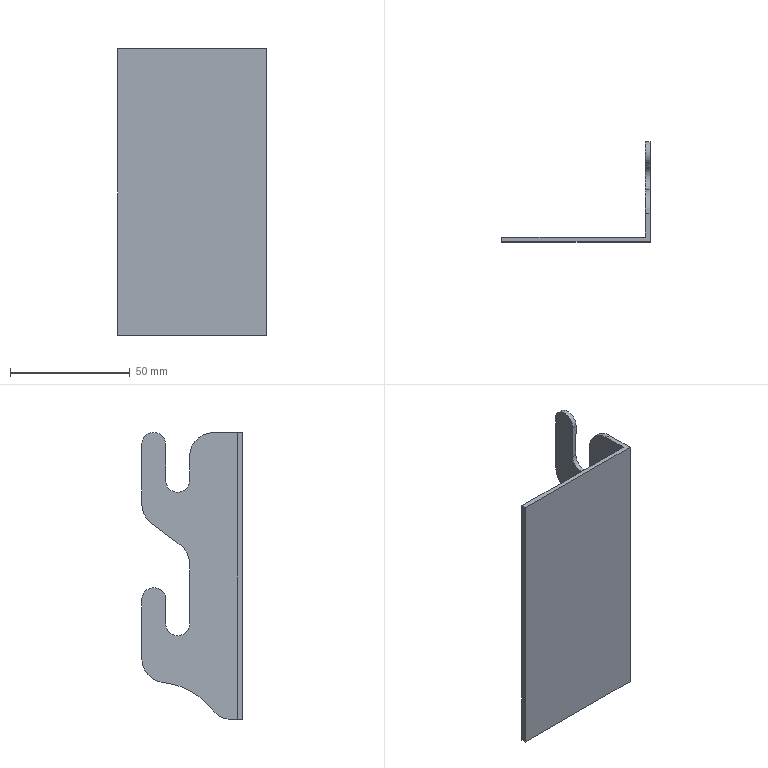Part | SolidWorks | features BaseBody 1 | 1 solid | 24 faces | box 62 x 42 x 120 mm | volume 21824 mm3 | plane 14 | cylinder 10 | commonest cylinder face diameters 20 x5 10 x3 10.188 x1 58.749 x1
STEP:
#1=CARTESIAN_POINT('',(-30.,2.,60.));
#2=VERTEX_POINT('',#1);
#3=CARTESIAN_POINT('',(30.,2.,60.));
#4=VERTEX_POINT('',#3);
#5=CARTESIAN_POINT('',(30.,2.,60.));
#6=DIRECTION('',(1.,0.,0.));
#7=VECTOR('',#6,1000.);
#8=LINE('',#5,#7);
#9=EDGE_CURVE('',#2,#4,#8,.T.);
#10=ORIENTED_EDGE('',*,*,#9,.T.);
#11=CARTESIAN_POINT('',(30.,2.,-60.));
#12=VERTEX_POINT('',#11);
#13=CARTESIAN_POINT('',(30.,2.,-60.));
#14=DIRECTION('',(0.,0.,-1.));
#15=VECTOR('',#14,1000.);
#16=LINE('',#13,#15);
#17=EDGE_CURVE('',#4,#12,#16,.T.);
#18=ORIENTED_EDGE('',*,*,#17,.T.);
#19=CARTESIAN_POINT('',(-30.,2.,-60.));
#20=VERTEX_POINT('',#19);
#21=CARTESIAN_POINT('',(-30.,2.,-60.));
#22=DIRECTION('',(-1.,0.,0.));
#23=VECTOR('',#22,1000.);
#24=LINE('',#21,#23);
#25=EDGE_CURVE('',#12,#20,#24,.T.);
#26=ORIENTED_EDGE('',*,*,#25,.T.);
#27=CARTESIAN_POINT('',(-30.,2.,60.));
#28=DIRECTION('',(0.,0.,1.));
#29=VECTOR('',#28,1000.);
#30=LINE('',#27,#29);
#31=EDGE_CURVE('',#20,#2,#30,.T.);
#32=ORIENTED_EDGE('',*,*,#31,.T.);
#33=EDGE_LOOP('',(#10,#18,#26,#32));
#34=FACE_OUTER_BOUND('',#33,.T.);
#35=CARTESIAN_POINT('',(0.,2.,0.));
#36=DIRECTION('',(0.,1.,0.));
#37=DIRECTION('',(1.,0.,0.));
#38=AXIS2_PLACEMENT_3D('',#35,#36,#37);
#39=PLANE('',#38);
#40=ADVANCED_FACE('',(#34),#39,.T.);
#41=CARTESIAN_POINT('',(32.,0.,60.));
#42=VERTEX_POINT('',#41);
#43=CARTESIAN_POINT('',(-30.,0.,60.));
#44=VERTEX_POINT('',#43);
#45=CARTESIAN_POINT('',(30.,0.,60.));
#46=DIRECTION('',(-1.,0.,0.));
#47=VECTOR('',#46,1000.);
#48=LINE('',#45,#47);
#49=EDGE_CURVE('',#42,#44,#48,.T.);
#50=ORIENTED_EDGE('',*,*,#49,.T.);
#51=CARTESIAN_POINT('',(-30.,0.,-60.));
#52=VERTEX_POINT('',#51);
#53=CARTESIAN_POINT('',(-30.,0.,60.));
#54=DIRECTION('',(0.,0.,-1.));
#55=VECTOR('',#54,1000.);
#56=LINE('',#53,#55);
#57=EDGE_CURVE('',#44,#52,#56,.T.);
#58=ORIENTED_EDGE('',*,*,#57,.T.);
#59=CARTESIAN_POINT('',(32.,0.,-60.));
#60=VERTEX_POINT('',#59);
#61=CARTESIAN_POINT('',(-30.,0.,-60.));
#62=DIRECTION('',(1.,0.,0.));
#63=VECTOR('',#62,1000.);
#64=LINE('',#61,#63);
#65=EDGE_CURVE('',#52,#60,#64,.T.);
#66=ORIENTED_EDGE('',*,*,#65,.T.);
#67=CARTESIAN_POINT('',(32.,0.,-60.));
#68=DIRECTION('',(0.,0.,-1.));
#69=VECTOR('',#68,1000.);
#70=LINE('',#67,#69);
#71=EDGE_CURVE('',#42,#60,#70,.T.);
#72=ORIENTED_EDGE('',*,*,#71,.F.);
#73=EDGE_LOOP('',(#50,#58,#66,#72));
#74=FACE_OUTER_BOUND('',#73,.T.);
#75=CARTESIAN_POINT('',(0.,0.,0.));
#76=DIRECTION('',(0.,-1.,0.));
#77=DIRECTION('',(0.,0.,-1.));
#78=AXIS2_PLACEMENT_3D('',#75,#76,#77);
#79=PLANE('',#78);
#80=ADVANCED_FACE('',(#74),#79,.T.);
#81=ORIENTED_EDGE('',*,*,#49,.F.);
#82=CARTESIAN_POINT('',(32.,12.,60.));
#83=VERTEX_POINT('',#82);
#84=CARTESIAN_POINT('',(32.,0.,60.));
#85=DIRECTION('',(0.,-1.,0.));
#86=VECTOR('',#85,1000.);
#87=LINE('',#84,#86);
#88=EDGE_CURVE('',#83,#42,#87,.T.);
#89=ORIENTED_EDGE('',*,*,#88,.F.);
#90=CARTESIAN_POINT('',(30.,12.,60.));
#91=VERTEX_POINT('',#90);
#92=CARTESIAN_POINT('',(30.,12.,60.));
#93=DIRECTION('',(1.,0.,0.));
#94=VECTOR('',#93,1000.);
#95=LINE('',#92,#94);
#96=EDGE_CURVE('',#91,#83,#95,.T.);
#97=ORIENTED_EDGE('',*,*,#96,.F.);
#98=CARTESIAN_POINT('',(30.,0.,60.));
#99=DIRECTION('',(0.,1.,0.));
#100=VECTOR('',#99,1000.);
#101=LINE('',#98,#100);
#102=EDGE_CURVE('',#4,#91,#101,.T.);
#103=ORIENTED_EDGE('',*,*,#102,.F.);
#104=ORIENTED_EDGE('',*,*,#9,.F.);
#105=CARTESIAN_POINT('',(-30.,0.,60.));
#106=DIRECTION('',(0.,1.,0.));
#107=VECTOR('',#106,1000.);
#108=LINE('',#105,#107);
#109=EDGE_CURVE('',#44,#2,#108,.T.);
#110=ORIENTED_EDGE('',*,*,#109,.F.);
#111=EDGE_LOOP('',(#81,#89,#97,#103,#104,#110));
#112=FACE_OUTER_BOUND('',#111,.T.);
#113=CARTESIAN_POINT('',(-30.,0.,60.));
#114=DIRECTION('',(0.,0.,1.));
#115=DIRECTION('',(1.,0.,0.));
#116=AXIS2_PLACEMENT_3D('',#113,#114,#115);
#117=PLANE('',#116);
#118=ADVANCED_FACE('',(#112),#117,.T.);
#119=ORIENTED_EDGE('',*,*,#65,.F.);
#120=CARTESIAN_POINT('',(-30.,0.,-60.));
#121=DIRECTION('',(0.,1.,0.));
#122=VECTOR('',#121,1000.);
#123=LINE('',#120,#122);
#124=EDGE_CURVE('',#52,#20,#123,.T.);
#125=ORIENTED_EDGE('',*,*,#124,.T.);
#126=ORIENTED_EDGE('',*,*,#25,.F.);
#127=CARTESIAN_POINT('',(30.,4.56,-60.));
#128=VERTEX_POINT('',#127);
#129=CARTESIAN_POINT('',(30.,4.56,-60.));
#130=DIRECTION('',(0.,-1.,0.));
#131=VECTOR('',#130,1000.);
#132=LINE('',#129,#131);
#133=EDGE_CURVE('',#128,#12,#132,.T.);
#134=ORIENTED_EDGE('',*,*,#133,.F.);
#135=CARTESIAN_POINT('',(32.,4.56,-60.));
#136=VERTEX_POINT('',#135);
#137=CARTESIAN_POINT('',(30.,4.56,-60.));
#138=DIRECTION('',(1.,0.,0.));
#139=VECTOR('',#138,1000.);
#140=LINE('',#137,#139);
#141=EDGE_CURVE('',#128,#136,#140,.T.);
#142=ORIENTED_EDGE('',*,*,#141,.T.);
#143=CARTESIAN_POINT('',(32.,4.56,-60.));
#144=DIRECTION('',(0.,1.,0.));
#145=VECTOR('',#144,1000.);
#146=LINE('',#143,#145);
#147=EDGE_CURVE('',#60,#136,#146,.T.);
#148=ORIENTED_EDGE('',*,*,#147,.F.);
#149=EDGE_LOOP('',(#119,#125,#126,#134,#142,#148));
#150=FACE_OUTER_BOUND('',#149,.T.);
#151=CARTESIAN_POINT('',(30.,0.,-60.));
#152=DIRECTION('',(0.,0.,-1.));
#153=DIRECTION('',(0.,-1.,0.));
#154=AXIS2_PLACEMENT_3D('',#151,#152,#153);
#155=PLANE('',#154);
#156=ADVANCED_FACE('',(#150),#155,.T.);
#157=ORIENTED_EDGE('',*,*,#57,.F.);
#158=ORIENTED_EDGE('',*,*,#109,.T.);
#159=ORIENTED_EDGE('',*,*,#31,.F.);
#160=ORIENTED_EDGE('',*,*,#124,.F.);
#161=EDGE_LOOP('',(#157,#158,#159,#160));
#162=FACE_OUTER_BOUND('',#161,.T.);
#163=CARTESIAN_POINT('',(-30.,0.,-60.));
#164=DIRECTION('',(-1.,0.,0.));
#165=DIRECTION('',(0.,1.,0.));
#166=AXIS2_PLACEMENT_3D('',#163,#164,#165);
#167=PLANE('',#166);
#168=ADVANCED_FACE('',(#162),#167,.T.);
#169=ORIENTED_EDGE('',*,*,#88,.T.);
#170=ORIENTED_EDGE('',*,*,#71,.T.);
#171=ORIENTED_EDGE('',*,*,#147,.T.);
#172=CARTESIAN_POINT('',(32.,12.53,-56.04));
#173=VERTEX_POINT('',#172);
#174=CARTESIAN_POINT('',(32.,4.56,-50.));
#175=DIRECTION('',(1.,0.,0.));
#176=DIRECTION('',(0.,0.,1.));
#177=AXIS2_PLACEMENT_3D('',#174,#175,#176);
#178=CIRCLE('',#177,10.);
#179=EDGE_CURVE('',#136,#173,#178,.T.);
#180=ORIENTED_EDGE('',*,*,#179,.T.);
#181=CARTESIAN_POINT('',(32.,33.001,-44.557));
#182=VERTEX_POINT('',#181);
#183=CARTESIAN_POINT('',(32.,35.94,-73.784));
#184=DIRECTION('',(-1.,0.,0.));
#185=DIRECTION('',(0.,-0.1001,0.995));
#186=AXIS2_PLACEMENT_3D('',#183,#184,#185);
#187=CIRCLE('',#186,29.374);
#188=EDGE_CURVE('',#173,#182,#187,.T.);
#189=ORIENTED_EDGE('',*,*,#188,.T.);
#190=CARTESIAN_POINT('',(32.,42.,-34.607));
#191=VERTEX_POINT('',#190);
#192=CARTESIAN_POINT('',(32.,32.,-34.607));
#193=DIRECTION('',(1.,0.,0.));
#194=DIRECTION('',(0.,-0.1001,0.995));
#195=AXIS2_PLACEMENT_3D('',#192,#193,#194);
#196=CIRCLE('',#195,10.);
#197=EDGE_CURVE('',#182,#191,#196,.T.);
#198=ORIENTED_EDGE('',*,*,#197,.T.);
#199=CARTESIAN_POINT('',(32.,42.,-10.));
#200=VERTEX_POINT('',#199);
#201=CARTESIAN_POINT('',(32.,42.,-10.));
#202=DIRECTION('',(0.,0.,1.));
#203=VECTOR('',#202,1000.);
#204=LINE('',#201,#203);
#205=EDGE_CURVE('',#191,#200,#204,.T.);
#206=ORIENTED_EDGE('',*,*,#205,.T.);
#207=CARTESIAN_POINT('',(32.,32.,-8.629));
#208=VERTEX_POINT('',#207);
#209=CARTESIAN_POINT('',(32.,36.906,-10.));
#210=DIRECTION('',(1.,0.,0.));
#211=DIRECTION('',(0.,-1.,0.));
#212=AXIS2_PLACEMENT_3D('',#209,#210,#211);
#213=CIRCLE('',#212,5.094);
#214=EDGE_CURVE('',#200,#208,#213,.T.);
#215=ORIENTED_EDGE('',*,*,#214,.T.);
#216=CARTESIAN_POINT('',(32.,32.,-20.));
#217=VERTEX_POINT('',#216);
#218=CARTESIAN_POINT('',(32.,32.,-20.));
#219=DIRECTION('',(0.,0.,-1.));
#220=VECTOR('',#219,1000.);
#221=LINE('',#218,#220);
#222=EDGE_CURVE('',#208,#217,#221,.T.);
#223=ORIENTED_EDGE('',*,*,#222,.T.);
#224=CARTESIAN_POINT('',(32.,22.,-20.));
#225=VERTEX_POINT('',#224);
#226=CARTESIAN_POINT('',(32.,27.,-20.));
#227=DIRECTION('',(-1.,0.,0.));
#228=DIRECTION('',(0.,-1.,0.));
#229=AXIS2_PLACEMENT_3D('',#226,#227,#228);
#230=CIRCLE('',#229,5.);
#231=EDGE_CURVE('',#217,#225,#230,.T.);
#232=ORIENTED_EDGE('',*,*,#231,.T.);
#233=CARTESIAN_POINT('',(32.,22.,5.051));
#234=VERTEX_POINT('',#233);
#235=CARTESIAN_POINT('',(32.,22.,5.051));
#236=DIRECTION('',(0.,0.,1.));
#237=VECTOR('',#236,1000.);
#238=LINE('',#235,#237);
#239=EDGE_CURVE('',#225,#234,#238,.T.);
#240=ORIENTED_EDGE('',*,*,#239,.T.);
#241=CARTESIAN_POINT('',(32.,26.,13.051));
#242=VERTEX_POINT('',#241);
#243=CARTESIAN_POINT('',(32.,32.,5.051));
#244=DIRECTION('',(-1.,0.,0.));
#245=DIRECTION('',(0.,-0.6,0.8));
#246=AXIS2_PLACEMENT_3D('',#243,#244,#245);
#247=CIRCLE('',#246,10.);
#248=EDGE_CURVE('',#234,#242,#247,.T.);
#249=ORIENTED_EDGE('',*,*,#248,.T.);
#250=CARTESIAN_POINT('',(32.,38.,22.051));
#251=VERTEX_POINT('',#250);
#252=CARTESIAN_POINT('',(32.,38.,22.051));
#253=DIRECTION('',(0.,0.8,0.6));
#254=VECTOR('',#253,1000.);
#255=LINE('',#252,#254);
#256=EDGE_CURVE('',#242,#251,#255,.T.);
#257=ORIENTED_EDGE('',*,*,#256,.T.);
#258=CARTESIAN_POINT('',(32.,42.,30.051));
#259=VERTEX_POINT('',#258);
#260=CARTESIAN_POINT('',(32.,32.,30.051));
#261=DIRECTION('',(1.,0.,0.));
#262=DIRECTION('',(0.,-0.6,0.8));
#263=AXIS2_PLACEMENT_3D('',#260,#261,#262);
#264=CIRCLE('',#263,10.);
#265=EDGE_CURVE('',#251,#259,#264,.T.);
#266=ORIENTED_EDGE('',*,*,#265,.T.);
#267=CARTESIAN_POINT('',(32.,42.,55.));
#268=VERTEX_POINT('',#267);
#269=CARTESIAN_POINT('',(32.,42.,55.));
#270=DIRECTION('',(0.,0.,1.));
#271=VECTOR('',#270,1000.);
#272=LINE('',#269,#271);
#273=EDGE_CURVE('',#259,#268,#272,.T.);
#274=ORIENTED_EDGE('',*,*,#273,.T.);
#275=CARTESIAN_POINT('',(32.,32.,55.));
#276=VERTEX_POINT('',#275);
#277=CARTESIAN_POINT('',(32.,37.,55.));
#278=DIRECTION('',(1.,0.,0.));
#279=DIRECTION('',(0.,-1.,0.));
#280=AXIS2_PLACEMENT_3D('',#277,#278,#279);
#281=CIRCLE('',#280,5.);
#282=EDGE_CURVE('',#268,#276,#281,.T.);
#283=ORIENTED_EDGE('',*,*,#282,.T.);
#284=CARTESIAN_POINT('',(32.,32.,40.));
#285=VERTEX_POINT('',#284);
#286=CARTESIAN_POINT('',(32.,32.,40.));
#287=DIRECTION('',(0.,0.,-1.));
#288=VECTOR('',#287,1000.);
#289=LINE('',#286,#288);
#290=EDGE_CURVE('',#276,#285,#289,.T.);
#291=ORIENTED_EDGE('',*,*,#290,.T.);
#292=CARTESIAN_POINT('',(32.,22.,40.));
#293=VERTEX_POINT('',#292);
#294=CARTESIAN_POINT('',(32.,27.,40.));
#295=DIRECTION('',(-1.,0.,0.));
#296=DIRECTION('',(0.,-1.,0.));
#297=AXIS2_PLACEMENT_3D('',#294,#295,#296);
#298=CIRCLE('',#297,5.);
#299=EDGE_CURVE('',#285,#293,#298,.T.);
#300=ORIENTED_EDGE('',*,*,#299,.T.);
#301=CARTESIAN_POINT('',(32.,22.,50.));
#302=VERTEX_POINT('',#301);
#303=CARTESIAN_POINT('',(32.,22.,50.));
#304=DIRECTION('',(0.,0.,1.));
#305=VECTOR('',#304,1000.);
#306=LINE('',#303,#305);
#307=EDGE_CURVE('',#293,#302,#306,.T.);
#308=ORIENTED_EDGE('',*,*,#307,.T.);
#309=CARTESIAN_POINT('',(32.,12.,50.));
#310=DIRECTION('',(1.,0.,0.));
#311=DIRECTION('',(0.,-1.,0.));
#312=AXIS2_PLACEMENT_3D('',#309,#310,#311);
#313=CIRCLE('',#312,10.);
#314=EDGE_CURVE('',#302,#83,#313,.T.);
#315=ORIENTED_EDGE('',*,*,#314,.T.);
#316=EDGE_LOOP('',(#169,#170,#171,#180,#189,#198,#206,#215,#223,#232,#240,#249,#257,#266,#274,#283,#291,#300,#308,#315));
#317=FACE_OUTER_BOUND('',#316,.T.);
#318=CARTESIAN_POINT('',(32.,19.668,5.335));
#319=DIRECTION('',(1.,0.,0.));
#320=DIRECTION('',(0.,0.,-1.));
#321=AXIS2_PLACEMENT_3D('',#318,#319,#320);
#322=PLANE('',#321);
#323=ADVANCED_FACE('',(#317),#322,.T.);
#324=ORIENTED_EDGE('',*,*,#17,.F.);
#325=ORIENTED_EDGE('',*,*,#102,.T.);
#326=CARTESIAN_POINT('',(30.,22.,50.));
#327=VERTEX_POINT('',#326);
#328=CARTESIAN_POINT('',(30.,12.,50.));
#329=DIRECTION('',(-1.,0.,0.));
#330=DIRECTION('',(0.,-1.,0.));
#331=AXIS2_PLACEMENT_3D('',#328,#329,#330);
#332=CIRCLE('',#331,10.);
#333=EDGE_CURVE('',#91,#327,#332,.T.);
#334=ORIENTED_EDGE('',*,*,#333,.T.);
#335=CARTESIAN_POINT('',(30.,22.,40.));
#336=VERTEX_POINT('',#335);
#337=CARTESIAN_POINT('',(30.,22.,50.));
#338=DIRECTION('',(0.,0.,-1.));
#339=VECTOR('',#338,1000.);
#340=LINE('',#337,#339);
#341=EDGE_CURVE('',#327,#336,#340,.T.);
#342=ORIENTED_EDGE('',*,*,#341,.T.);
#343=CARTESIAN_POINT('',(30.,32.,40.));
#344=VERTEX_POINT('',#343);
#345=CARTESIAN_POINT('',(30.,27.,40.));
#346=DIRECTION('',(1.,0.,0.));
#347=DIRECTION('',(0.,-1.,0.));
#348=AXIS2_PLACEMENT_3D('',#345,#346,#347);
#349=CIRCLE('',#348,5.);
#350=EDGE_CURVE('',#336,#344,#349,.T.);
#351=ORIENTED_EDGE('',*,*,#350,.T.);
#352=CARTESIAN_POINT('',(30.,32.,55.));
#353=VERTEX_POINT('',#352);
#354=CARTESIAN_POINT('',(30.,32.,40.));
#355=DIRECTION('',(0.,0.,1.));
#356=VECTOR('',#355,1000.);
#357=LINE('',#354,#356);
#358=EDGE_CURVE('',#344,#353,#357,.T.);
#359=ORIENTED_EDGE('',*,*,#358,.T.);
#360=CARTESIAN_POINT('',(30.,42.,55.));
#361=VERTEX_POINT('',#360);
#362=CARTESIAN_POINT('',(30.,37.,55.));
#363=DIRECTION('',(-1.,0.,0.));
#364=DIRECTION('',(0.,-1.,0.));
#365=AXIS2_PLACEMENT_3D('',#362,#363,#364);
#366=CIRCLE('',#365,5.);
#367=EDGE_CURVE('',#353,#361,#366,.T.);
#368=ORIENTED_EDGE('',*,*,#367,.T.);
#369=CARTESIAN_POINT('',(30.,42.,30.051));
#370=VERTEX_POINT('',#369);
#371=CARTESIAN_POINT('',(30.,42.,55.));
#372=DIRECTION('',(0.,0.,-1.));
#373=VECTOR('',#372,1000.);
#374=LINE('',#371,#373);
#375=EDGE_CURVE('',#361,#370,#374,.T.);
#376=ORIENTED_EDGE('',*,*,#375,.T.);
#377=CARTESIAN_POINT('',(30.,38.,22.051));
#378=VERTEX_POINT('',#377);
#379=CARTESIAN_POINT('',(30.,32.,30.051));
#380=DIRECTION('',(-1.,0.,0.));
#381=DIRECTION('',(0.,-0.6,0.8));
#382=AXIS2_PLACEMENT_3D('',#379,#380,#381);
#383=CIRCLE('',#382,10.);
#384=EDGE_CURVE('',#370,#378,#383,.T.);
#385=ORIENTED_EDGE('',*,*,#384,.T.);
#386=CARTESIAN_POINT('',(30.,26.,13.051));
#387=VERTEX_POINT('',#386);
#388=CARTESIAN_POINT('',(30.,38.,22.051));
#389=DIRECTION('',(0.,-0.8,-0.6));
#390=VECTOR('',#389,1000.);
#391=LINE('',#388,#390);
#392=EDGE_CURVE('',#378,#387,#391,.T.);
#393=ORIENTED_EDGE('',*,*,#392,.T.);
#394=CARTESIAN_POINT('',(30.,22.,5.051));
#395=VERTEX_POINT('',#394);
#396=CARTESIAN_POINT('',(30.,32.,5.051));
#397=DIRECTION('',(1.,0.,0.));
#398=DIRECTION('',(0.,-0.6,0.8));
#399=AXIS2_PLACEMENT_3D('',#396,#397,#398);
#400=CIRCLE('',#399,10.);
#401=EDGE_CURVE('',#387,#395,#400,.T.);
#402=ORIENTED_EDGE('',*,*,#401,.T.);
#403=CARTESIAN_POINT('',(30.,22.,-20.));
#404=VERTEX_POINT('',#403);
#405=CARTESIAN_POINT('',(30.,22.,5.051));
#406=DIRECTION('',(0.,0.,-1.));
#407=VECTOR('',#406,1000.);
#408=LINE('',#405,#407);
#409=EDGE_CURVE('',#395,#404,#408,.T.);
#410=ORIENTED_EDGE('',*,*,#409,.T.);
#411=CARTESIAN_POINT('',(30.,32.,-20.));
#412=VERTEX_POINT('',#411);
#413=CARTESIAN_POINT('',(30.,27.,-20.));
#414=DIRECTION('',(1.,0.,0.));
#415=DIRECTION('',(0.,-1.,0.));
#416=AXIS2_PLACEMENT_3D('',#413,#414,#415);
#417=CIRCLE('',#416,5.);
#418=EDGE_CURVE('',#404,#412,#417,.T.);
#419=ORIENTED_EDGE('',*,*,#418,.T.);
#420=CARTESIAN_POINT('',(30.,32.,-8.629));
#421=VERTEX_POINT('',#420);
#422=CARTESIAN_POINT('',(30.,32.,-20.));
#423=DIRECTION('',(0.,0.,1.));
#424=VECTOR('',#423,1000.);
#425=LINE('',#422,#424);
#426=EDGE_CURVE('',#412,#421,#425,.T.);
#427=ORIENTED_EDGE('',*,*,#426,.T.);
#428=CARTESIAN_POINT('',(30.,42.,-10.));
#429=VERTEX_POINT('',#428);
#430=CARTESIAN_POINT('',(30.,36.906,-10.));
#431=DIRECTION('',(-1.,0.,0.));
#432=DIRECTION('',(0.,-1.,0.));
#433=AXIS2_PLACEMENT_3D('',#430,#431,#432);
#434=CIRCLE('',#433,5.094);
#435=EDGE_CURVE('',#421,#429,#434,.T.);
#436=ORIENTED_EDGE('',*,*,#435,.T.);
#437=CARTESIAN_POINT('',(30.,42.,-34.607));
#438=VERTEX_POINT('',#437);
#439=CARTESIAN_POINT('',(30.,42.,-10.));
#440=DIRECTION('',(0.,0.,-1.));
#441=VECTOR('',#440,1000.);
#442=LINE('',#439,#441);
#443=EDGE_CURVE('',#429,#438,#442,.T.);
#444=ORIENTED_EDGE('',*,*,#443,.T.);
#445=CARTESIAN_POINT('',(30.,33.001,-44.557));
#446=VERTEX_POINT('',#445);
#447=CARTESIAN_POINT('',(30.,32.,-34.607));
#448=DIRECTION('',(-1.,0.,0.));
#449=DIRECTION('',(0.,-0.1001,0.995));
#450=AXIS2_PLACEMENT_3D('',#447,#448,#449);
#451=CIRCLE('',#450,10.);
#452=EDGE_CURVE('',#438,#446,#451,.T.);
#453=ORIENTED_EDGE('',*,*,#452,.T.);
#454=CARTESIAN_POINT('',(30.,12.53,-56.04));
#455=VERTEX_POINT('',#454);
#456=CARTESIAN_POINT('',(30.,35.94,-73.784));
#457=DIRECTION('',(1.,0.,0.));
#458=DIRECTION('',(0.,-0.1001,0.995));
#459=AXIS2_PLACEMENT_3D('',#456,#457,#458);
#460=CIRCLE('',#459,29.374);
#461=EDGE_CURVE('',#446,#455,#460,.T.);
#462=ORIENTED_EDGE('',*,*,#461,.T.);
#463=CARTESIAN_POINT('',(30.,4.56,-50.));
#464=DIRECTION('',(-1.,0.,0.));
#465=DIRECTION('',(0.,0.,1.));
#466=AXIS2_PLACEMENT_3D('',#463,#464,#465);
#467=CIRCLE('',#466,10.);
#468=EDGE_CURVE('',#455,#128,#467,.T.);
#469=ORIENTED_EDGE('',*,*,#468,.T.);
#470=ORIENTED_EDGE('',*,*,#133,.T.);
#471=EDGE_LOOP('',(#324,#325,#334,#342,#351,#359,#368,#376,#385,#393,#402,#410,#419,#427,#436,#444,#453,#462,#469,#470));
#472=FACE_OUTER_BOUND('',#471,.T.);
#473=CARTESIAN_POINT('',(30.,19.668,5.335));
#474=DIRECTION('',(1.,0.,0.));
#475=DIRECTION('',(0.,0.,-1.));
#476=AXIS2_PLACEMENT_3D('',#473,#474,#475);
#477=PLANE('',#476);
#478=ADVANCED_FACE('',(#472),#477,.F.);
#479=ORIENTED_EDGE('',*,*,#468,.F.);
#480=CARTESIAN_POINT('',(30.,12.53,-56.04));
#481=DIRECTION('',(1.,0.,0.));
#482=VECTOR('',#481,1000.);
#483=LINE('',#480,#482);
#484=EDGE_CURVE('',#455,#173,#483,.T.);
#485=ORIENTED_EDGE('',*,*,#484,.T.);
#486=ORIENTED_EDGE('',*,*,#179,.F.);
#487=ORIENTED_EDGE('',*,*,#141,.F.);
#488=EDGE_LOOP('',(#479,#485,#486,#487));
#489=FACE_OUTER_BOUND('',#488,.T.);
#490=CARTESIAN_POINT('',(30.,4.56,-50.));
#491=DIRECTION('',(1.,0.,0.));
#492=DIRECTION('',(0.,0.,1.));
#493=AXIS2_PLACEMENT_3D('',#490,#491,#492);
#494=CYLINDRICAL_SURFACE('',#493,10.);
#495=ADVANCED_FACE('',(#489),#494,.T.);
#496=ORIENTED_EDGE('',*,*,#461,.F.);
#497=CARTESIAN_POINT('',(30.,33.001,-44.557));
#498=DIRECTION('',(1.,0.,0.));
#499=VECTOR('',#498,1000.);
#500=LINE('',#497,#499);
#501=EDGE_CURVE('',#446,#182,#500,.T.);
#502=ORIENTED_EDGE('',*,*,#501,.T.);
#503=ORIENTED_EDGE('',*,*,#188,.F.);
#504=ORIENTED_EDGE('',*,*,#484,.F.);
#505=EDGE_LOOP('',(#496,#502,#503,#504));
#506=FACE_OUTER_BOUND('',#505,.T.);
#507=CARTESIAN_POINT('',(30.,35.94,-73.784));
#508=DIRECTION('',(1.,0.,0.));
#509=DIRECTION('',(0.,-0.1001,0.995));
#510=AXIS2_PLACEMENT_3D('',#507,#508,#509);
#511=CYLINDRICAL_SURFACE('',#510,29.374);
#512=ADVANCED_FACE('',(#506),#511,.F.);
#513=ORIENTED_EDGE('',*,*,#452,.F.);
#514=CARTESIAN_POINT('',(30.,42.,-34.607));
#515=DIRECTION('',(1.,0.,0.));
#516=VECTOR('',#515,1000.);
#517=LINE('',#514,#516);
#518=EDGE_CURVE('',#438,#191,#517,.T.);
#519=ORIENTED_EDGE('',*,*,#518,.T.);
#520=ORIENTED_EDGE('',*,*,#197,.F.);
#521=ORIENTED_EDGE('',*,*,#501,.F.);
#522=EDGE_LOOP('',(#513,#519,#520,#521));
#523=FACE_OUTER_BOUND('',#522,.T.);
#524=CARTESIAN_POINT('',(30.,32.,-34.607));
#525=DIRECTION('',(1.,0.,0.));
#526=DIRECTION('',(0.,-0.1001,0.995));
#527=AXIS2_PLACEMENT_3D('',#524,#525,#526);
#528=CYLINDRICAL_SURFACE('',#527,10.);
#529=ADVANCED_FACE('',(#523),#528,.T.);
#530=ORIENTED_EDGE('',*,*,#443,.F.);
#531=CARTESIAN_POINT('',(30.,42.,-10.));
#532=DIRECTION('',(1.,0.,0.));
#533=VECTOR('',#532,1000.);
#534=LINE('',#531,#533);
#535=EDGE_CURVE('',#429,#200,#534,.T.);
#536=ORIENTED_EDGE('',*,*,#535,.T.);
#537=ORIENTED_EDGE('',*,*,#205,.F.);
#538=ORIENTED_EDGE('',*,*,#518,.F.);
#539=EDGE_LOOP('',(#530,#536,#537,#538));
#540=FACE_OUTER_BOUND('',#539,.T.);
#541=CARTESIAN_POINT('',(30.,42.,-34.607));
#542=DIRECTION('',(0.,1.,0.));
#543=DIRECTION('',(0.,0.,-1.));
#544=AXIS2_PLACEMENT_3D('',#541,#542,#543);
#545=PLANE('',#544);
#546=ADVANCED_FACE('',(#540),#545,.T.);
#547=ORIENTED_EDGE('',*,*,#435,.F.);
#548=CARTESIAN_POINT('',(30.,32.,-8.629));
#549=DIRECTION('',(1.,0.,0.));
#550=VECTOR('',#549,1000.);
#551=LINE('',#548,#550);
#552=EDGE_CURVE('',#421,#208,#551,.T.);
#553=ORIENTED_EDGE('',*,*,#552,.T.);
#554=ORIENTED_EDGE('',*,*,#214,.F.);
#555=ORIENTED_EDGE('',*,*,#535,.F.);
#556=EDGE_LOOP('',(#547,#553,#554,#555));
#557=FACE_OUTER_BOUND('',#556,.T.);
#558=CARTESIAN_POINT('',(30.,36.906,-10.));
#559=DIRECTION('',(1.,0.,0.));
#560=DIRECTION('',(0.,-1.,0.));
#561=AXIS2_PLACEMENT_3D('',#558,#559,#560);
#562=CYLINDRICAL_SURFACE('',#561,5.094);
#563=ADVANCED_FACE('',(#557),#562,.T.);
#564=ORIENTED_EDGE('',*,*,#426,.F.);
#565=CARTESIAN_POINT('',(30.,32.,-20.));
#566=DIRECTION('',(1.,0.,0.));
#567=VECTOR('',#566,1000.);
#568=LINE('',#565,#567);
#569=EDGE_CURVE('',#412,#217,#568,.T.);
#570=ORIENTED_EDGE('',*,*,#569,.T.);
#571=ORIENTED_EDGE('',*,*,#222,.F.);
#572=ORIENTED_EDGE('',*,*,#552,.F.);
#573=EDGE_LOOP('',(#564,#570,#571,#572));
#574=FACE_OUTER_BOUND('',#573,.T.);
#575=CARTESIAN_POINT('',(30.,32.,-8.629));
#576=DIRECTION('',(0.,-1.,0.));
#577=DIRECTION('',(0.,0.,-1.));
#578=AXIS2_PLACEMENT_3D('',#575,#576,#577);
#579=PLANE('',#578);
#580=ADVANCED_FACE('',(#574),#579,.T.);
#581=ORIENTED_EDGE('',*,*,#418,.F.);
#582=CARTESIAN_POINT('',(30.,22.,-20.));
#583=DIRECTION('',(1.,0.,0.));
#584=VECTOR('',#583,1000.);
#585=LINE('',#582,#584);
#586=EDGE_CURVE('',#404,#225,#585,.T.);
#587=ORIENTED_EDGE('',*,*,#586,.T.);
#588=ORIENTED_EDGE('',*,*,#231,.F.);
#589=ORIENTED_EDGE('',*,*,#569,.F.);
#590=EDGE_LOOP('',(#581,#587,#588,#589));
#591=FACE_OUTER_BOUND('',#590,.T.);
#592=CARTESIAN_POINT('',(30.,27.,-20.));
#593=DIRECTION('',(1.,0.,0.));
#594=DIRECTION('',(0.,-1.,0.));
#595=AXIS2_PLACEMENT_3D('',#592,#593,#594);
#596=CYLINDRICAL_SURFACE('',#595,5.);
#597=ADVANCED_FACE('',(#591),#596,.F.);
#598=ORIENTED_EDGE('',*,*,#409,.F.);
#599=CARTESIAN_POINT('',(30.,22.,5.051));
#600=DIRECTION('',(1.,0.,0.));
#601=VECTOR('',#600,1000.);
#602=LINE('',#599,#601);
#603=EDGE_CURVE('',#395,#234,#602,.T.);
#604=ORIENTED_EDGE('',*,*,#603,.T.);
#605=ORIENTED_EDGE('',*,*,#239,.F.);
#606=ORIENTED_EDGE('',*,*,#586,.F.);
#607=EDGE_LOOP('',(#598,#604,#605,#606));
#608=FACE_OUTER_BOUND('',#607,.T.);
#609=CARTESIAN_POINT('',(30.,22.,-20.));
#610=DIRECTION('',(0.,1.,0.));
#611=DIRECTION('',(0.,0.,-1.));
#612=AXIS2_PLACEMENT_3D('',#609,#610,#611);
#613=PLANE('',#612);
#614=ADVANCED_FACE('',(#608),#613,.T.);
#615=ORIENTED_EDGE('',*,*,#401,.F.);
#616=CARTESIAN_POINT('',(30.,26.,13.051));
#617=DIRECTION('',(1.,0.,0.));
#618=VECTOR('',#617,1000.);
#619=LINE('',#616,#618);
#620=EDGE_CURVE('',#387,#242,#619,.T.);
#621=ORIENTED_EDGE('',*,*,#620,.T.);
#622=ORIENTED_EDGE('',*,*,#248,.F.);
#623=ORIENTED_EDGE('',*,*,#603,.F.);
#624=EDGE_LOOP('',(#615,#621,#622,#623));
#625=FACE_OUTER_BOUND('',#624,.T.);
#626=CARTESIAN_POINT('',(30.,32.,5.051));
#627=DIRECTION('',(1.,0.,0.));
#628=DIRECTION('',(0.,-0.6,0.8));
#629=AXIS2_PLACEMENT_3D('',#626,#627,#628);
#630=CYLINDRICAL_SURFACE('',#629,10.);
#631=ADVANCED_FACE('',(#625),#630,.F.);
#632=ORIENTED_EDGE('',*,*,#392,.F.);
#633=CARTESIAN_POINT('',(30.,38.,22.051));
#634=DIRECTION('',(1.,0.,0.));
#635=VECTOR('',#634,1000.);
#636=LINE('',#633,#635);
#637=EDGE_CURVE('',#378,#251,#636,.T.);
#638=ORIENTED_EDGE('',*,*,#637,.T.);
#639=ORIENTED_EDGE('',*,*,#256,.F.);
#640=ORIENTED_EDGE('',*,*,#620,.F.);
#641=EDGE_LOOP('',(#632,#638,#639,#640));
#642=FACE_OUTER_BOUND('',#641,.T.);
#643=CARTESIAN_POINT('',(30.,26.,13.051));
#644=DIRECTION('',(0.,0.6,-0.8));
#645=DIRECTION('',(-1.,0.,0.));
#646=AXIS2_PLACEMENT_3D('',#643,#644,#645);
#647=PLANE('',#646);
#648=ADVANCED_FACE('',(#642),#647,.T.);
#649=ORIENTED_EDGE('',*,*,#384,.F.);
#650=CARTESIAN_POINT('',(30.,42.,30.051));
#651=DIRECTION('',(1.,0.,0.));
#652=VECTOR('',#651,1000.);
#653=LINE('',#650,#652);
#654=EDGE_CURVE('',#370,#259,#653,.T.);
#655=ORIENTED_EDGE('',*,*,#654,.T.);
#656=ORIENTED_EDGE('',*,*,#265,.F.);
#657=ORIENTED_EDGE('',*,*,#637,.F.);
#658=EDGE_LOOP('',(#649,#655,#656,#657));
#659=FACE_OUTER_BOUND('',#658,.T.);
#660=CARTESIAN_POINT('',(30.,32.,30.051));
#661=DIRECTION('',(1.,0.,0.));
#662=DIRECTION('',(0.,-0.6,0.8));
#663=AXIS2_PLACEMENT_3D('',#660,#661,#662);
#664=CYLINDRICAL_SURFACE('',#663,10.);
#665=ADVANCED_FACE('',(#659),#664,.T.);
#666=ORIENTED_EDGE('',*,*,#375,.F.);
#667=CARTESIAN_POINT('',(30.,42.,55.));
#668=DIRECTION('',(1.,0.,0.));
#669=VECTOR('',#668,1000.);
#670=LINE('',#667,#669);
#671=EDGE_CURVE('',#361,#268,#670,.T.);
#672=ORIENTED_EDGE('',*,*,#671,.T.);
#673=ORIENTED_EDGE('',*,*,#273,.F.);
#674=ORIENTED_EDGE('',*,*,#654,.F.);
#675=EDGE_LOOP('',(#666,#672,#673,#674));
#676=FACE_OUTER_BOUND('',#675,.T.);
#677=CARTESIAN_POINT('',(30.,42.,30.051));
#678=DIRECTION('',(0.,1.,0.));
#679=DIRECTION('',(1.,0.,0.));
#680=AXIS2_PLACEMENT_3D('',#677,#678,#679);
#681=PLANE('',#680);
#682=ADVANCED_FACE('',(#676),#681,.T.);
#683=ORIENTED_EDGE('',*,*,#367,.F.);
#684=CARTESIAN_POINT('',(30.,32.,55.));
#685=DIRECTION('',(1.,0.,0.));
#686=VECTOR('',#685,1000.);
#687=LINE('',#684,#686);
#688=EDGE_CURVE('',#353,#276,#687,.T.);
#689=ORIENTED_EDGE('',*,*,#688,.T.);
#690=ORIENTED_EDGE('',*,*,#282,.F.);
#691=ORIENTED_EDGE('',*,*,#671,.F.);
#692=EDGE_LOOP('',(#683,#689,#690,#691));
#693=FACE_OUTER_BOUND('',#692,.T.);
#694=CARTESIAN_POINT('',(30.,37.,55.));
#695=DIRECTION('',(1.,0.,0.));
#696=DIRECTION('',(0.,-1.,0.));
#697=AXIS2_PLACEMENT_3D('',#694,#695,#696);
#698=CYLINDRICAL_SURFACE('',#697,5.);
#699=ADVANCED_FACE('',(#693),#698,.T.);
#700=ORIENTED_EDGE('',*,*,#358,.F.);
#701=CARTESIAN_POINT('',(30.,32.,40.));
#702=DIRECTION('',(1.,0.,0.));
#703=VECTOR('',#702,1000.);
#704=LINE('',#701,#703);
#705=EDGE_CURVE('',#344,#285,#704,.T.);
#706=ORIENTED_EDGE('',*,*,#705,.T.);
#707=ORIENTED_EDGE('',*,*,#290,.F.);
#708=ORIENTED_EDGE('',*,*,#688,.F.);
#709=EDGE_LOOP('',(#700,#706,#707,#708));
#710=FACE_OUTER_BOUND('',#709,.T.);
#711=CARTESIAN_POINT('',(30.,32.,55.));
#712=DIRECTION('',(0.,-1.,0.));
#713=DIRECTION('',(0.,0.,-1.));
#714=AXIS2_PLACEMENT_3D('',#711,#712,#713);
#715=PLANE('',#714);
#716=ADVANCED_FACE('',(#710),#715,.T.);
#717=ORIENTED_EDGE('',*,*,#350,.F.);
#718=CARTESIAN_POINT('',(30.,22.,40.));
#719=DIRECTION('',(1.,0.,0.));
#720=VECTOR('',#719,1000.);
#721=LINE('',#718,#720);
#722=EDGE_CURVE('',#336,#293,#721,.T.);
#723=ORIENTED_EDGE('',*,*,#722,.T.);
#724=ORIENTED_EDGE('',*,*,#299,.F.);
#725=ORIENTED_EDGE('',*,*,#705,.F.);
#726=EDGE_LOOP('',(#717,#723,#724,#725));
#727=FACE_OUTER_BOUND('',#726,.T.);
#728=CARTESIAN_POINT('',(30.,27.,40.));
#729=DIRECTION('',(1.,0.,0.));
#730=DIRECTION('',(0.,-1.,0.));
#731=AXIS2_PLACEMENT_3D('',#728,#729,#730);
#732=CYLINDRICAL_SURFACE('',#731,5.);
#733=ADVANCED_FACE('',(#727),#732,.F.);
#734=ORIENTED_EDGE('',*,*,#341,.F.);
#735=CARTESIAN_POINT('',(30.,22.,50.));
#736=DIRECTION('',(1.,0.,0.));
#737=VECTOR('',#736,1000.);
#738=LINE('',#735,#737);
#739=EDGE_CURVE('',#327,#302,#738,.T.);
#740=ORIENTED_EDGE('',*,*,#739,.T.);
#741=ORIENTED_EDGE('',*,*,#307,.F.);
#742=ORIENTED_EDGE('',*,*,#722,.F.);
#743=EDGE_LOOP('',(#734,#740,#741,#742));
#744=FACE_OUTER_BOUND('',#743,.T.);
#745=CARTESIAN_POINT('',(30.,22.,40.));
#746=DIRECTION('',(0.,1.,0.));
#747=DIRECTION('',(1.,0.,0.));
#748=AXIS2_PLACEMENT_3D('',#745,#746,#747);
#749=PLANE('',#748);
#750=ADVANCED_FACE('',(#744),#749,.T.);
#751=ORIENTED_EDGE('',*,*,#333,.F.);
#752=ORIENTED_EDGE('',*,*,#96,.T.);
#753=ORIENTED_EDGE('',*,*,#314,.F.);
#754=ORIENTED_EDGE('',*,*,#739,.F.);
#755=EDGE_LOOP('',(#751,#752,#753,#754));
#756=FACE_OUTER_BOUND('',#755,.T.);
#757=CARTESIAN_POINT('',(30.,12.,50.));
#758=DIRECTION('',(1.,0.,0.));
#759=DIRECTION('',(0.,-1.,0.));
#760=AXIS2_PLACEMENT_3D('',#757,#758,#759);
#761=CYLINDRICAL_SURFACE('',#760,10.);
#762=ADVANCED_FACE('',(#756),#761,.T.);
#763=CLOSED_SHELL('',(#40,#80,#118,#156,#168,#323,#478,#495,#512,#529,#546,#563,#580,#597,#614,#631,#648,#665,#682,#699,#716,#733,#750,#762));
#764=MANIFOLD_SOLID_BREP('',#763);
#765=CARTESIAN_POINT('',(0.,0.,0.));
#766=DIRECTION('',(0.,0.,1.));
#767=DIRECTION('',(1.,0.,0.));
#768=AXIS2_PLACEMENT_3D('',#765,#766,#767);
#769=(LENGTH_UNIT()NAMED_UNIT(*)SI_UNIT(.MILLI.,.METRE.));
#770=UNCERTAINTY_MEASURE_WITH_UNIT(LENGTH_MEASURE(0.00001),#769,'','');
#771=(NAMED_UNIT(*)PLANE_ANGLE_UNIT()SI_UNIT($,.RADIAN.));
#772=(NAMED_UNIT(*)SI_UNIT($,.STERADIAN.)SOLID_ANGLE_UNIT());
#773=(GEOMETRIC_REPRESENTATION_CONTEXT(3)GLOBAL_UNCERTAINTY_ASSIGNED_CONTEXT((#770))GLOBAL_UNIT_ASSIGNED_CONTEXT((#769,#771,#772))REPRESENTATION_CONTEXT('',''));
#774=ADVANCED_BREP_SHAPE_REPRESENTATION('',(#764,#768),#773);